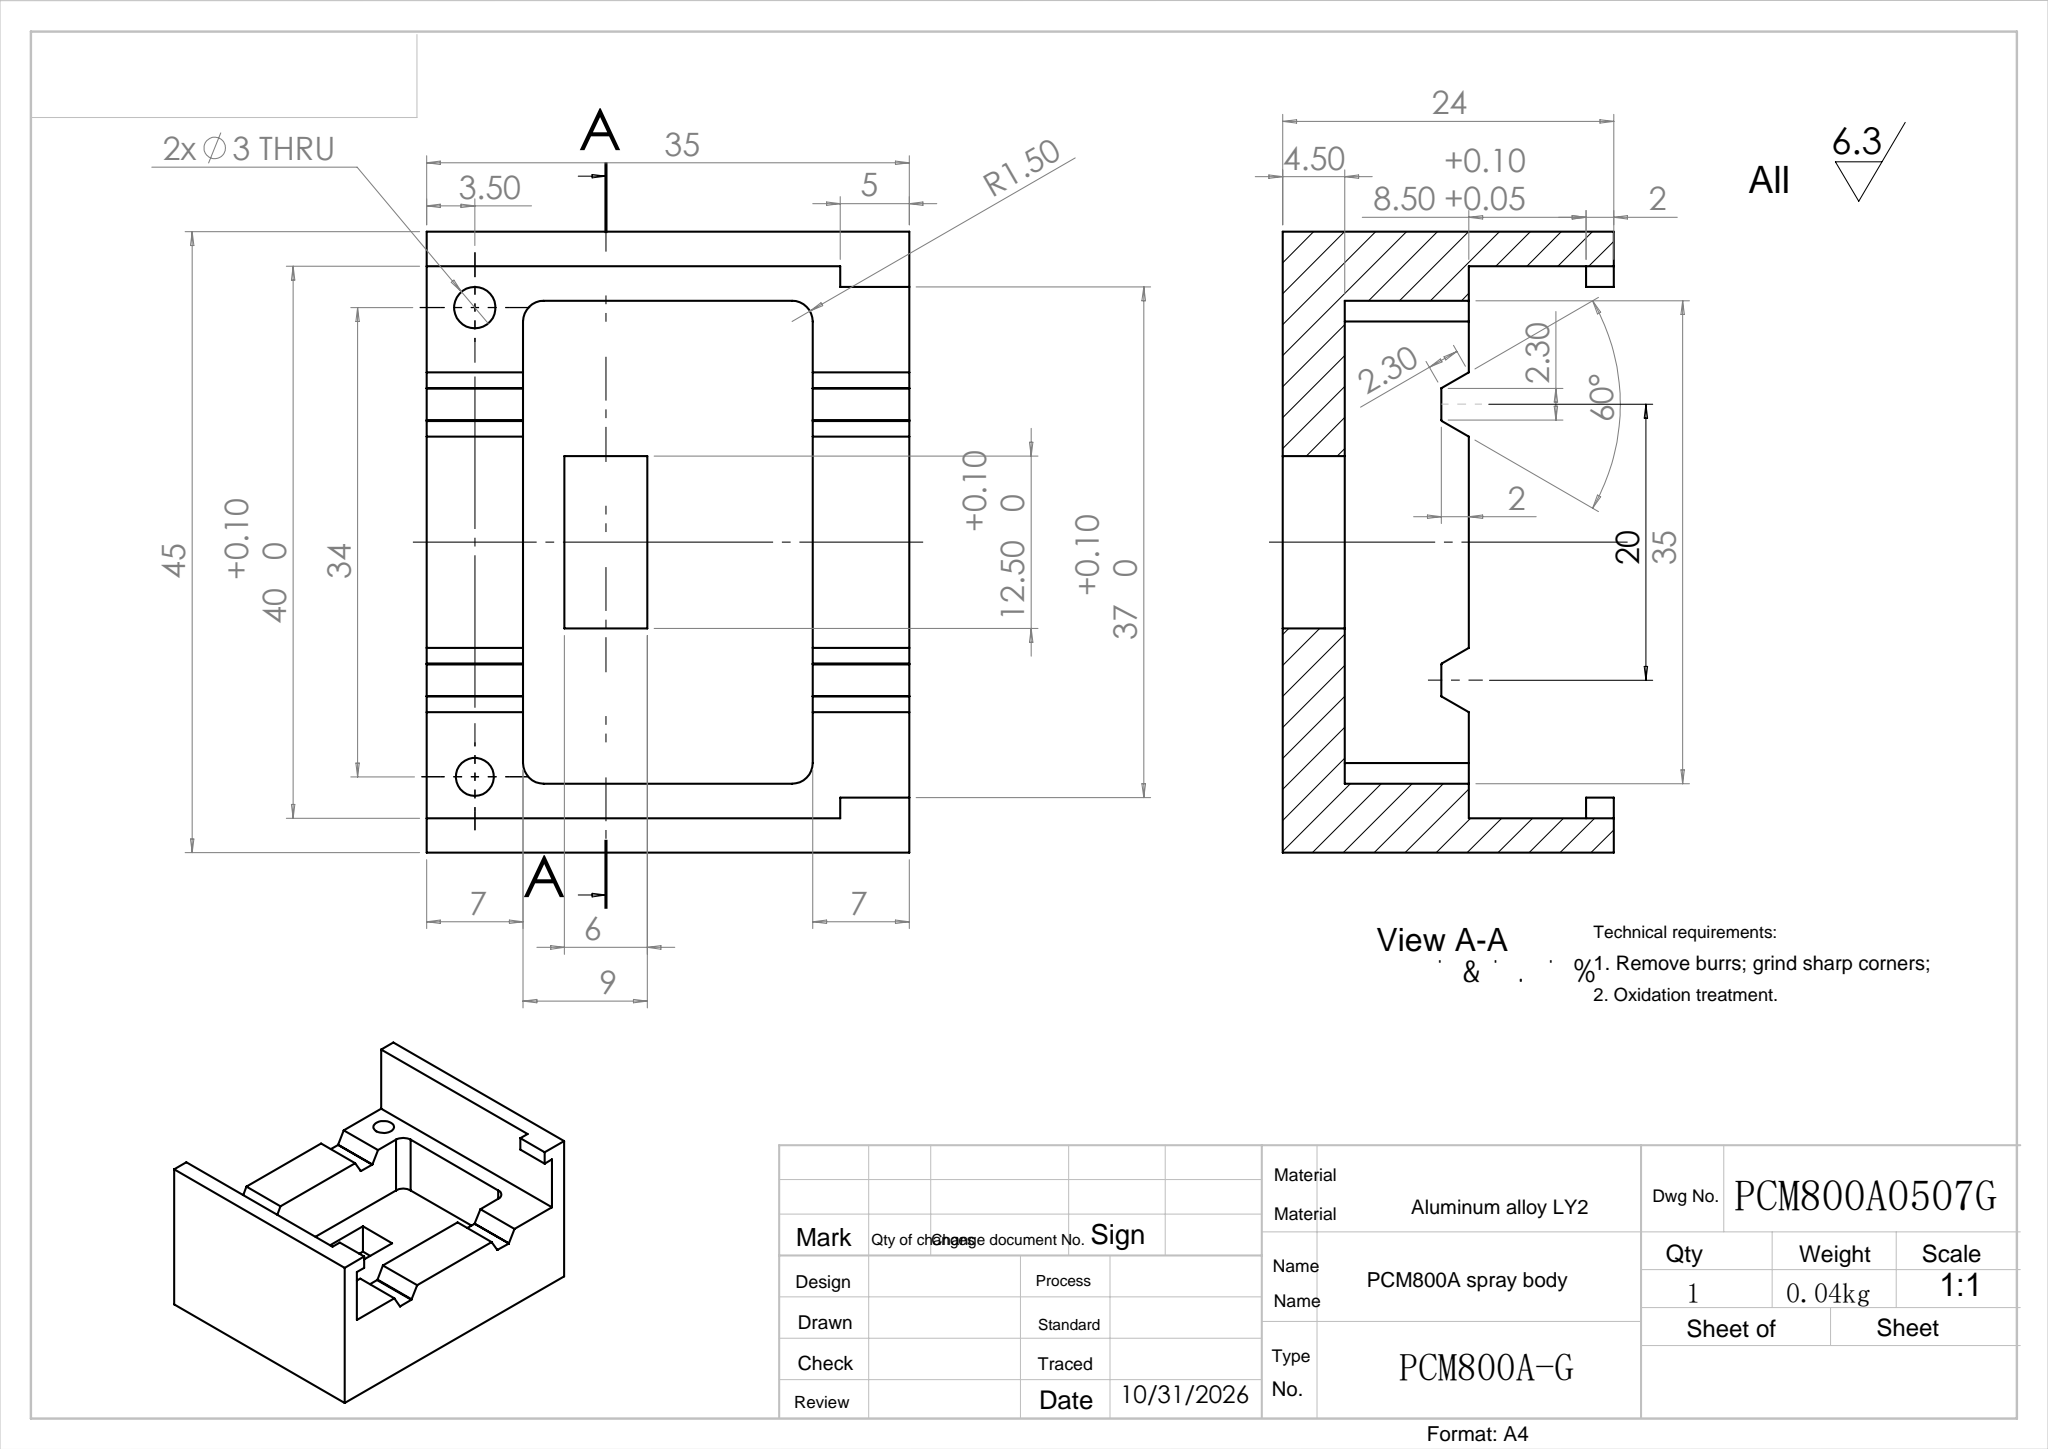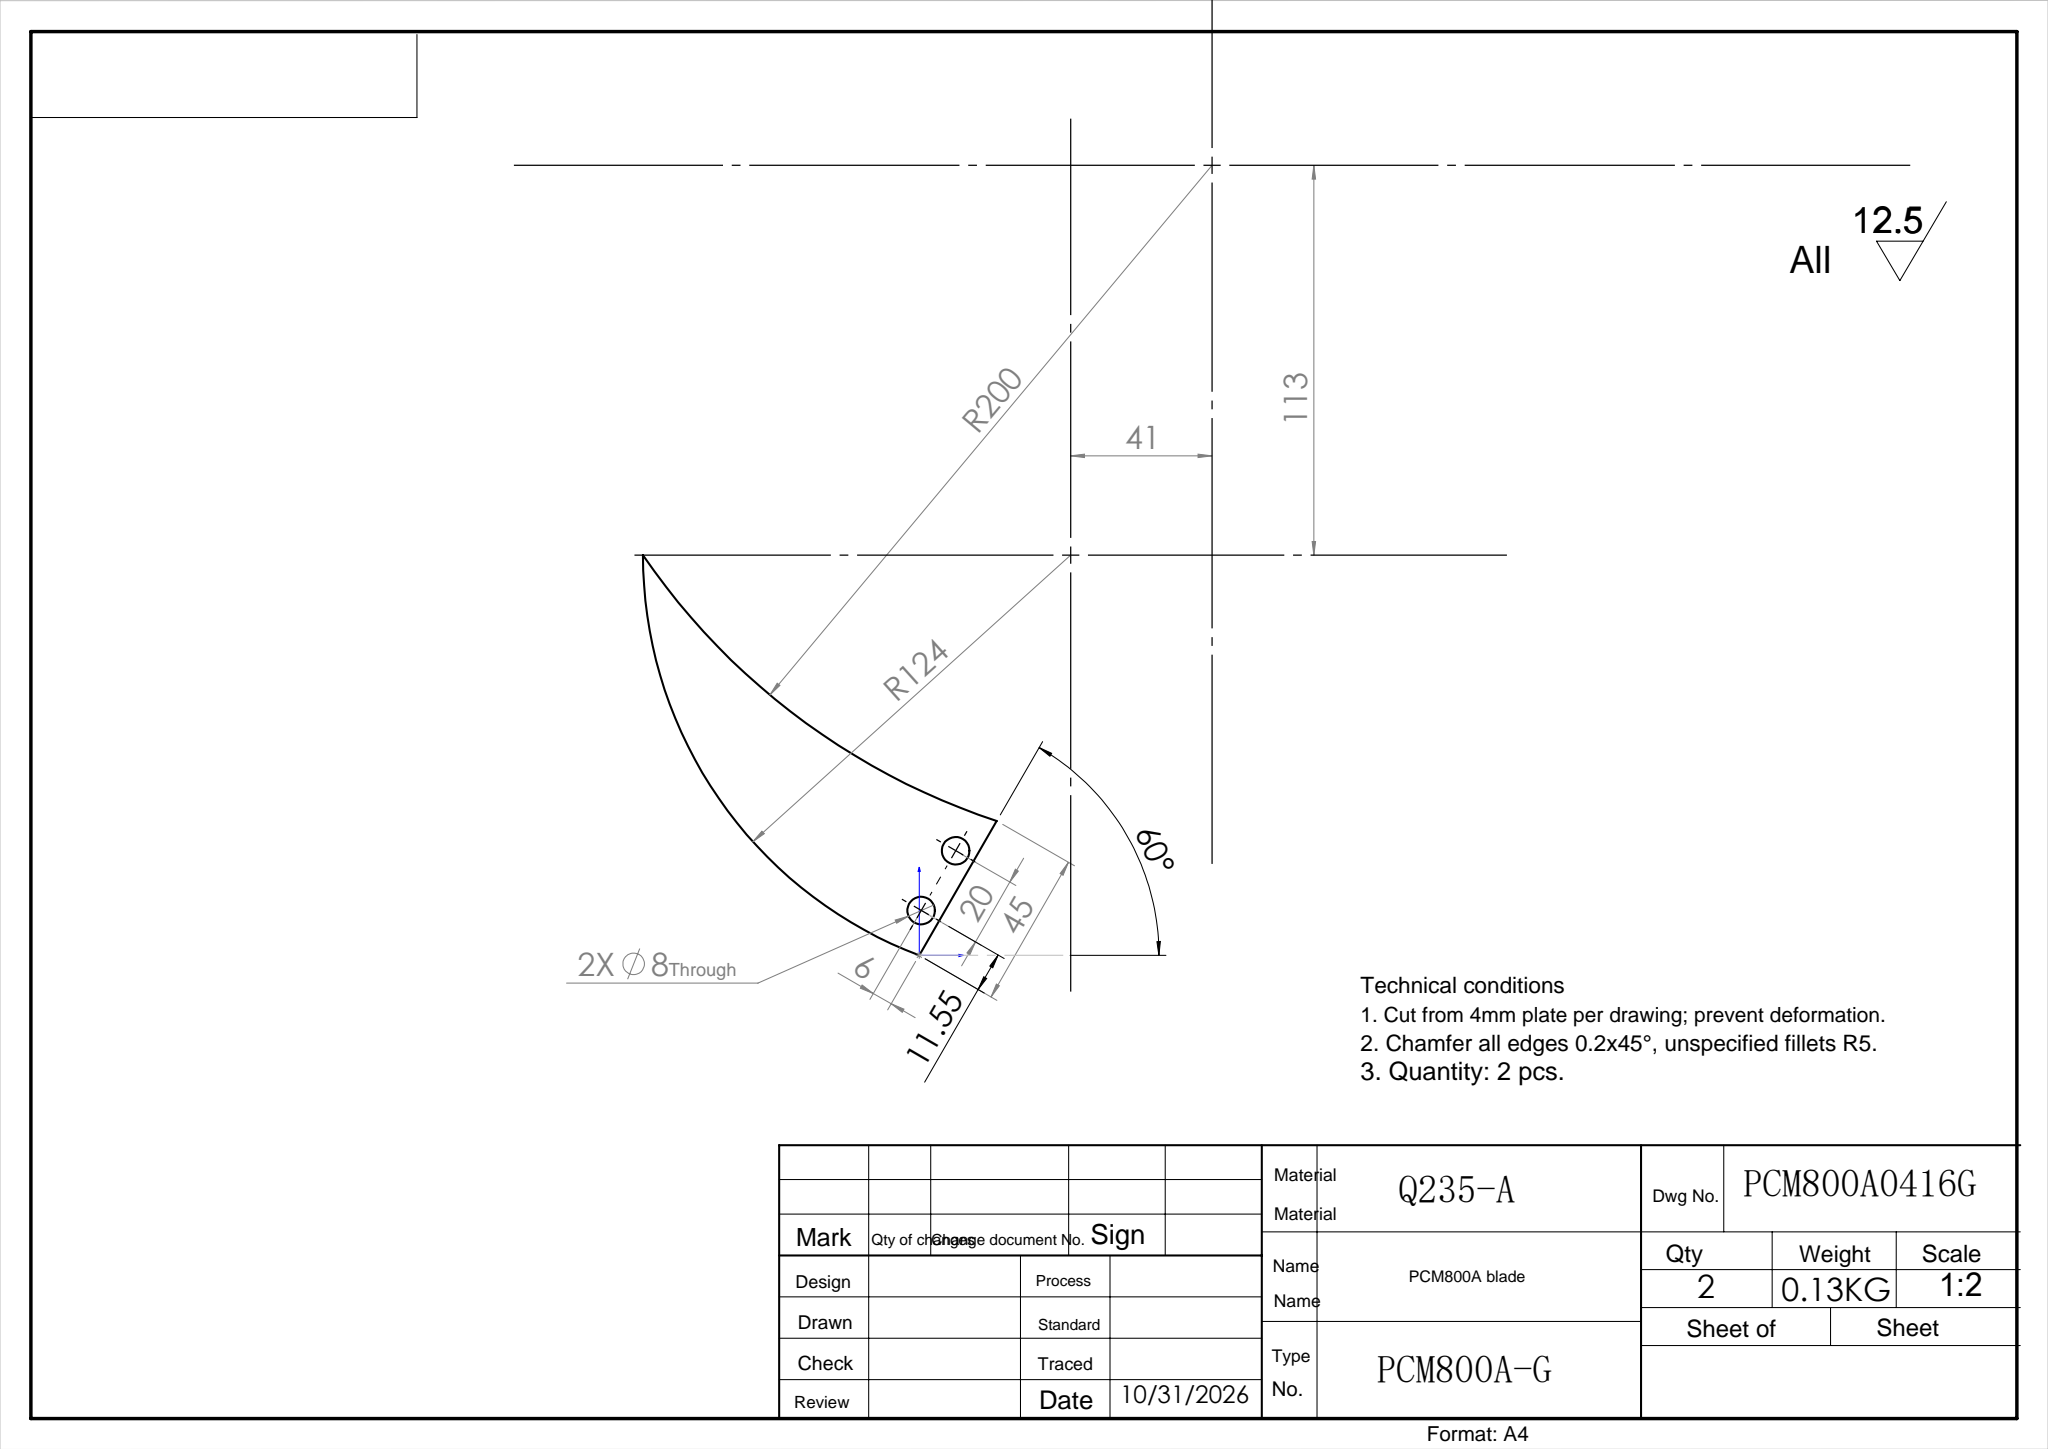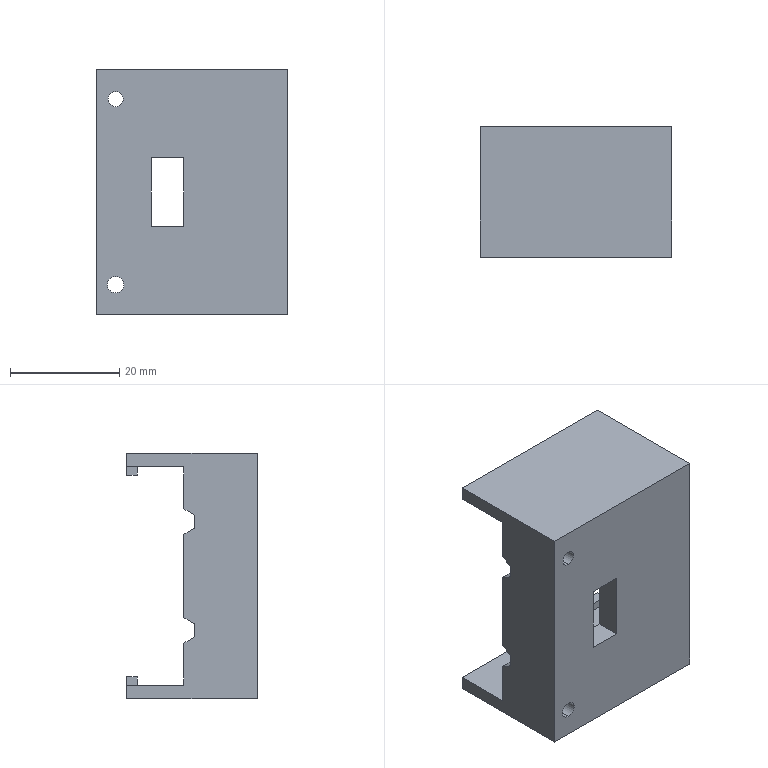Part | SolidWorks | features Cut 6, Boss 2, MirrorPattern 2, Extrusion 1, Fillet 1 | 1 solid | 56 faces | box 35 x 24 x 45 mm | volume 15822 mm3 | plane 48 | cylinder 8 | commonest cylinder face diameters 3 x4 2.757 x2 2.998 x2